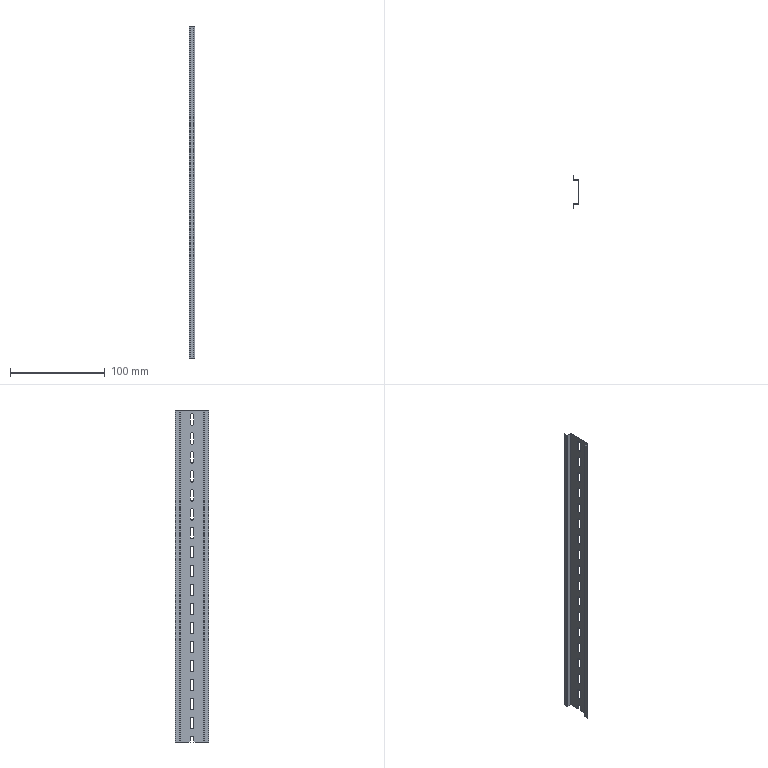Part | STEP file | 1 solid | 110 faces | box 5.5 x 35 x 350 mm | volume 7332 mm3 | plane 67 | cylinder 43 | commonest cylinder face diameters 4.2 x35 0.4 x4 1.4 x4